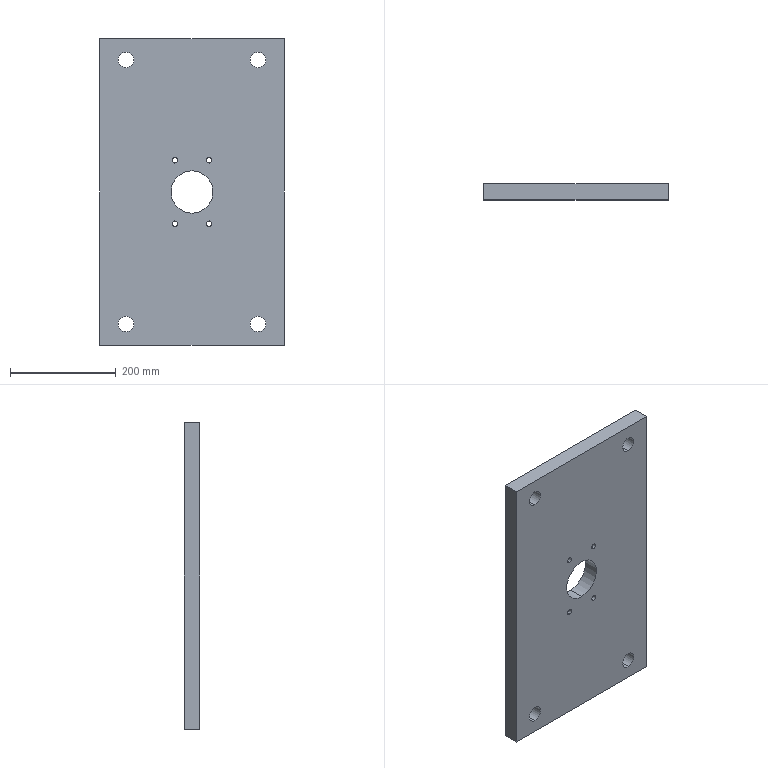Part | STEP file | 1 solid | 40 faces | box 350 x 30 x 580 mm | volume 5843358 mm3 | cylinder 26 | cone 8 | plane 6 | commonest cylinder face diameters 5 x8 10.2 x8 30 x8 80 x2